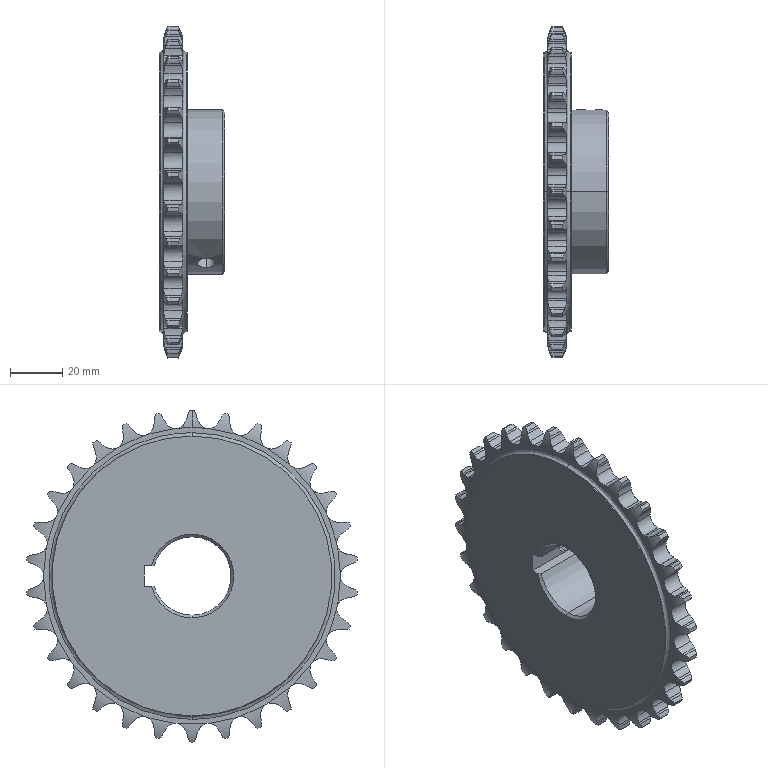Part | STEP file | PN_0014_driving sprocket_05B | 1 solid | 353 faces | box 25 x 126.465 x 127 mm | volume 135337 mm3 | cylinder 210 | plane 69 | spline 66 | cone 8 | commonest cylinder face diameters 11.344 x64 20.732 x64 8.06 x38 127 x31 6.8 x4 107 x4